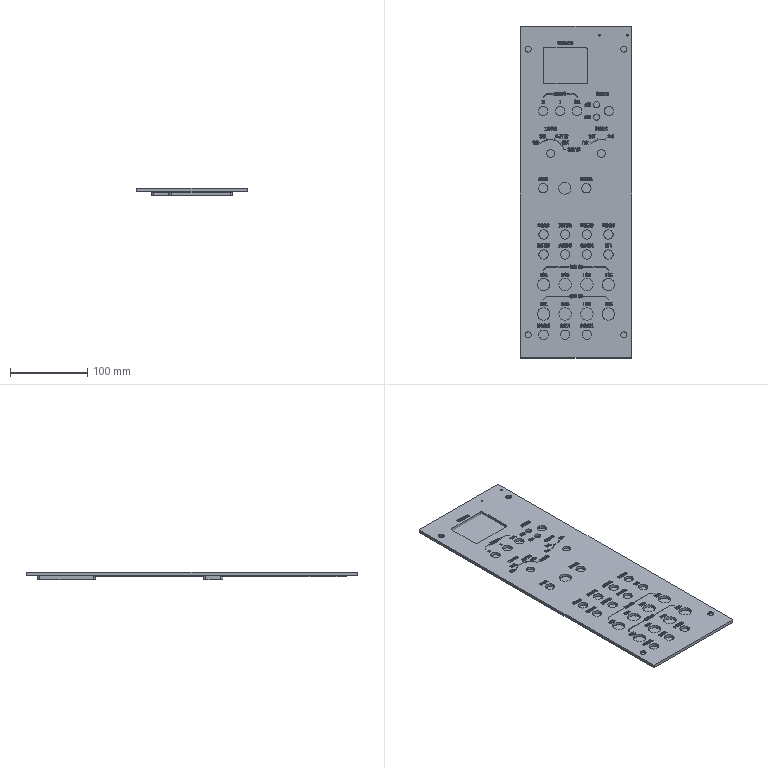CAM job | Mastercam | 3-axis milling, 5-axis milling, drilling | stock box 150 x 435 x 10 mm
Tools:
tool_number,name,type,diameter_mm,corner_radius_mm,flutes,flute_length_mm,overall_length_mm,shoulder_length_mm,holder_diameter_mm,length_offset,diameter_offset,default_rpm,default_feed_mm_min,default_plunge_mm_min,coolant
2,2 Flat End Mill,end mill,2,0,4,25,75,25,50,2,2,10000,2000,600,COOL_OFF
3,3 Flat End Mill,end mill,3,0,4,25,75,25,50,3,3,10000,3000,600,COOL_OFF
4,4 Flat End Mill,end mill,4,0,4,25,75,25,50,4,4,7000,3000,600,COOL_OFF
5,4 Chamfer Mill,chamfer mill,4,0,4,25,75,30,50,5,5,3000,300,600,COOL_OFF
9,10 Flat End Mill,end mill,10,0,4,25,75,25,50,9,9,7000,3000,600,COOL_OFF
10,10 Flat End Mill,end mill,10,0,4,25,75,25,50,10,10,7000,1000,600,COOL_OFF
Operations:
seq,operation,operation_type,tool_number,tool_name,tool_diameter_mm,spindle_rpm,feed_mm_min,plunge_mm_min,retract_mm_min,cycle_time_s,wcs,posted,nc_file
1,Contour (Ramp) - [WCS: Plane] - [Tplane: Plane],Contour,9,10 Flat End Mill,10,7000,3000,600,1200,259.286,Plane,yes,.nc
2,3D High Speed (Area roughing) - [WCS: Plane] - [Tplane: Plane],HighSpeed3D,9,10 Flat End Mill,10,7000,4000,600,1200,2433.299,Plane,yes,.nc
3,2D High Speed (2D Area Mill) - [WCS: Plane] - [Tplane: Plane],HighSpeed2D,9,10 Flat End Mill,10,7000,3000,600,1200,29.039,Plane,yes,.nc
4,Contour (2D) - [WCS: Plane] - [Tplane: Plane],Contour,10,10 Flat End Mill,10,7000,1000,600,1200,12.816,Plane,yes,.nc
5,Contour (2D) - [WCS: Plane] - [Tplane: Plane],Contour,10,10 Flat End Mill,10,7000,1000,600,1200,72.708,Plane,yes,.nc
6,3D High Speed (Waterline rest passes) - [WCS: Plane] - [Tplane: Plane],HighSpeed3D,4,4 Flat End Mill,4,7000,3000,600,1200,50.552,Plane,yes,.nc
7,3D High Speed (Horizontal) - [WCS: Plane] - [Tplane: Plane],HighSpeed3D,4,4 Flat End Mill,4,7000,1000,600,1200,1885.508,Plane,yes,.nc
8,3D High Speed (Waterline) - [WCS: Plane] - [Tplane: Plane],HighSpeed3D,4,4 Flat End Mill,4,7000,800,600,1200,250.531,Plane,yes,.nc
9,Surface Finish Flowline - [WCS: Plane] - [Tplane: Plane],MultiSurfaceFinishFlowline,4,4 Flat End Mill,4,50000,3000,600,1200,113.916,Plane,yes,.nc
10,Contour (Ramp) - [WCS: Plane] - [Tplane: Plane],Contour,4,4 Flat End Mill,4,10000,3000,600,1200,118.921,Plane,yes,.nc
11,Contour (Ramp) - [WCS: Plane] - [Tplane: Plane],Contour,4,4 Flat End Mill,4,10000,3000,600,1200,16.586,Plane,yes,.nc
12,Contour (Ramp) - [WCS: Plane] - [Tplane: Plane],Contour,3,3 Flat End Mill,3,10000,1000,600,1200,53.823,Plane,yes,.nc
13,Contour (Ramp) - [WCS: Plane] - [Tplane: Plane],Contour,3,3 Flat End Mill,3,10000,1000,600,1200,9.187,Plane,yes,.nc
14,Contour (2D) - [WCS: Plane] - [Tplane: Plane],Contour,3,3 Flat End Mill,3,10000,500,600,1200,3.476,Plane,yes,.nc
15,Contour (Ramp) - [WCS: Plane] - [Tplane: Plane],Contour,3,3 Flat End Mill,3,10000,3000,600,1200,15.729,Plane,yes,.nc
16,Contour (Ramp) - [WCS: Plane] - [Tplane: Plane],Contour,3,3 Flat End Mill,3,10000,3000,600,1200,306.348,Plane,yes,.nc
17,2D High Speed (2D Area Mill) - [WCS: Plane] - [Tplane: Plane],HighSpeed2D,2,2 Flat End Mill,2,10000,2000,600,1200,51.364,Plane,yes,.nc
18,2D High Speed (2D Area Mill) - [WCS: Plane] - [Tplane: Plane],HighSpeed2D,2,2 Flat End Mill,2,10000,800,600,1200,24.601,Plane,yes,.nc
19,Contour (Ramp) - [WCS: Plane] - [Tplane: Plane],Contour,2,2 Flat End Mill,2,10000,2000,600,1200,4.688,Plane,yes,.nc
20,Contour (2D) - [WCS: Plane] - [Tplane: Plane],Contour,2,2 Flat End Mill,2,10000,500,600,1200,2.772,Plane,yes,.nc
21,Contour (Ramp) - [WCS: Plane] - [Tplane: Plane],Contour,2,2 Flat End Mill,2,10000,2000,600,1200,43.14,Plane,yes,.nc
22,Contour (2D) - [WCS: Plane] - [Tplane: Plane],Contour,2,2 Flat End Mill,2,10000,500,600,1200,17.77,Plane,yes,.nc
23,2D High Speed (2D Area Mill) - [WCS: Plane] - [Tplane: Plane],HighSpeed2D,2,2 Flat End Mill,2,10000,500,600,1200,12.738,Plane,yes,.nc
24,Contour (Ramp) - [WCS: Plane] - [Tplane: Plane],Contour,3,3 Flat End Mill,3,10000,800,600,1200,9.05,Plane,yes,.nc
25,Contour (Ramp) - [WCS: Plane] - [Tplane: Plane],Contour,3,3 Flat End Mill,3,10000,800,600,1200,137.177,Plane,yes,.nc
26,Drill/Counterbore - [WCS: Plane] - [Tplane: Plane],Drill,5,4 Chamfer Mill,4,3000,300,600,1200,9.489,Plane,yes,.nc
27,Deburr 5-axis - [WCS: Plane] - [Tplane: Plane],459,5,4 Chamfer Mill,4,7000,1000,600,1200,404.136,Plane,yes,.nc
28,Contour (2D chamfer) - [WCS: Plane-1] - [Tplane: Plane-1],Contour,5,4 Chamfer Mill,4,7000,1000,600,1200,176.595,Plane-1,yes,.nc
29,Contour (2D) - [WCS: Plane-1] - [Tplane: Plane-1],Contour,4,4 Flat End Mill,4,7000,3000,600,1200,65.68,Plane-1,yes,.nc
30,Contour (2D) - [WCS: Plane-1] - [Tplane: Plane-1],Contour,4,4 Flat End Mill,4,7000,500,600,1200,10.476,Plane-1,yes,.nc
31,Helix Bore - [WCS: Plane-1] - [Tplane: Plane-1],HelixBore,3,3 Flat End Mill,3,7000,2000,600,1200,5.318,Plane-1,yes,.nc
32,Model Chamfer - [WCS: Plane-1] - [Tplane: Plane-1],ModelChamfer,5,4 Chamfer Mill,4,7000,1000,600,1200,6.73,Plane-1,yes,.nc